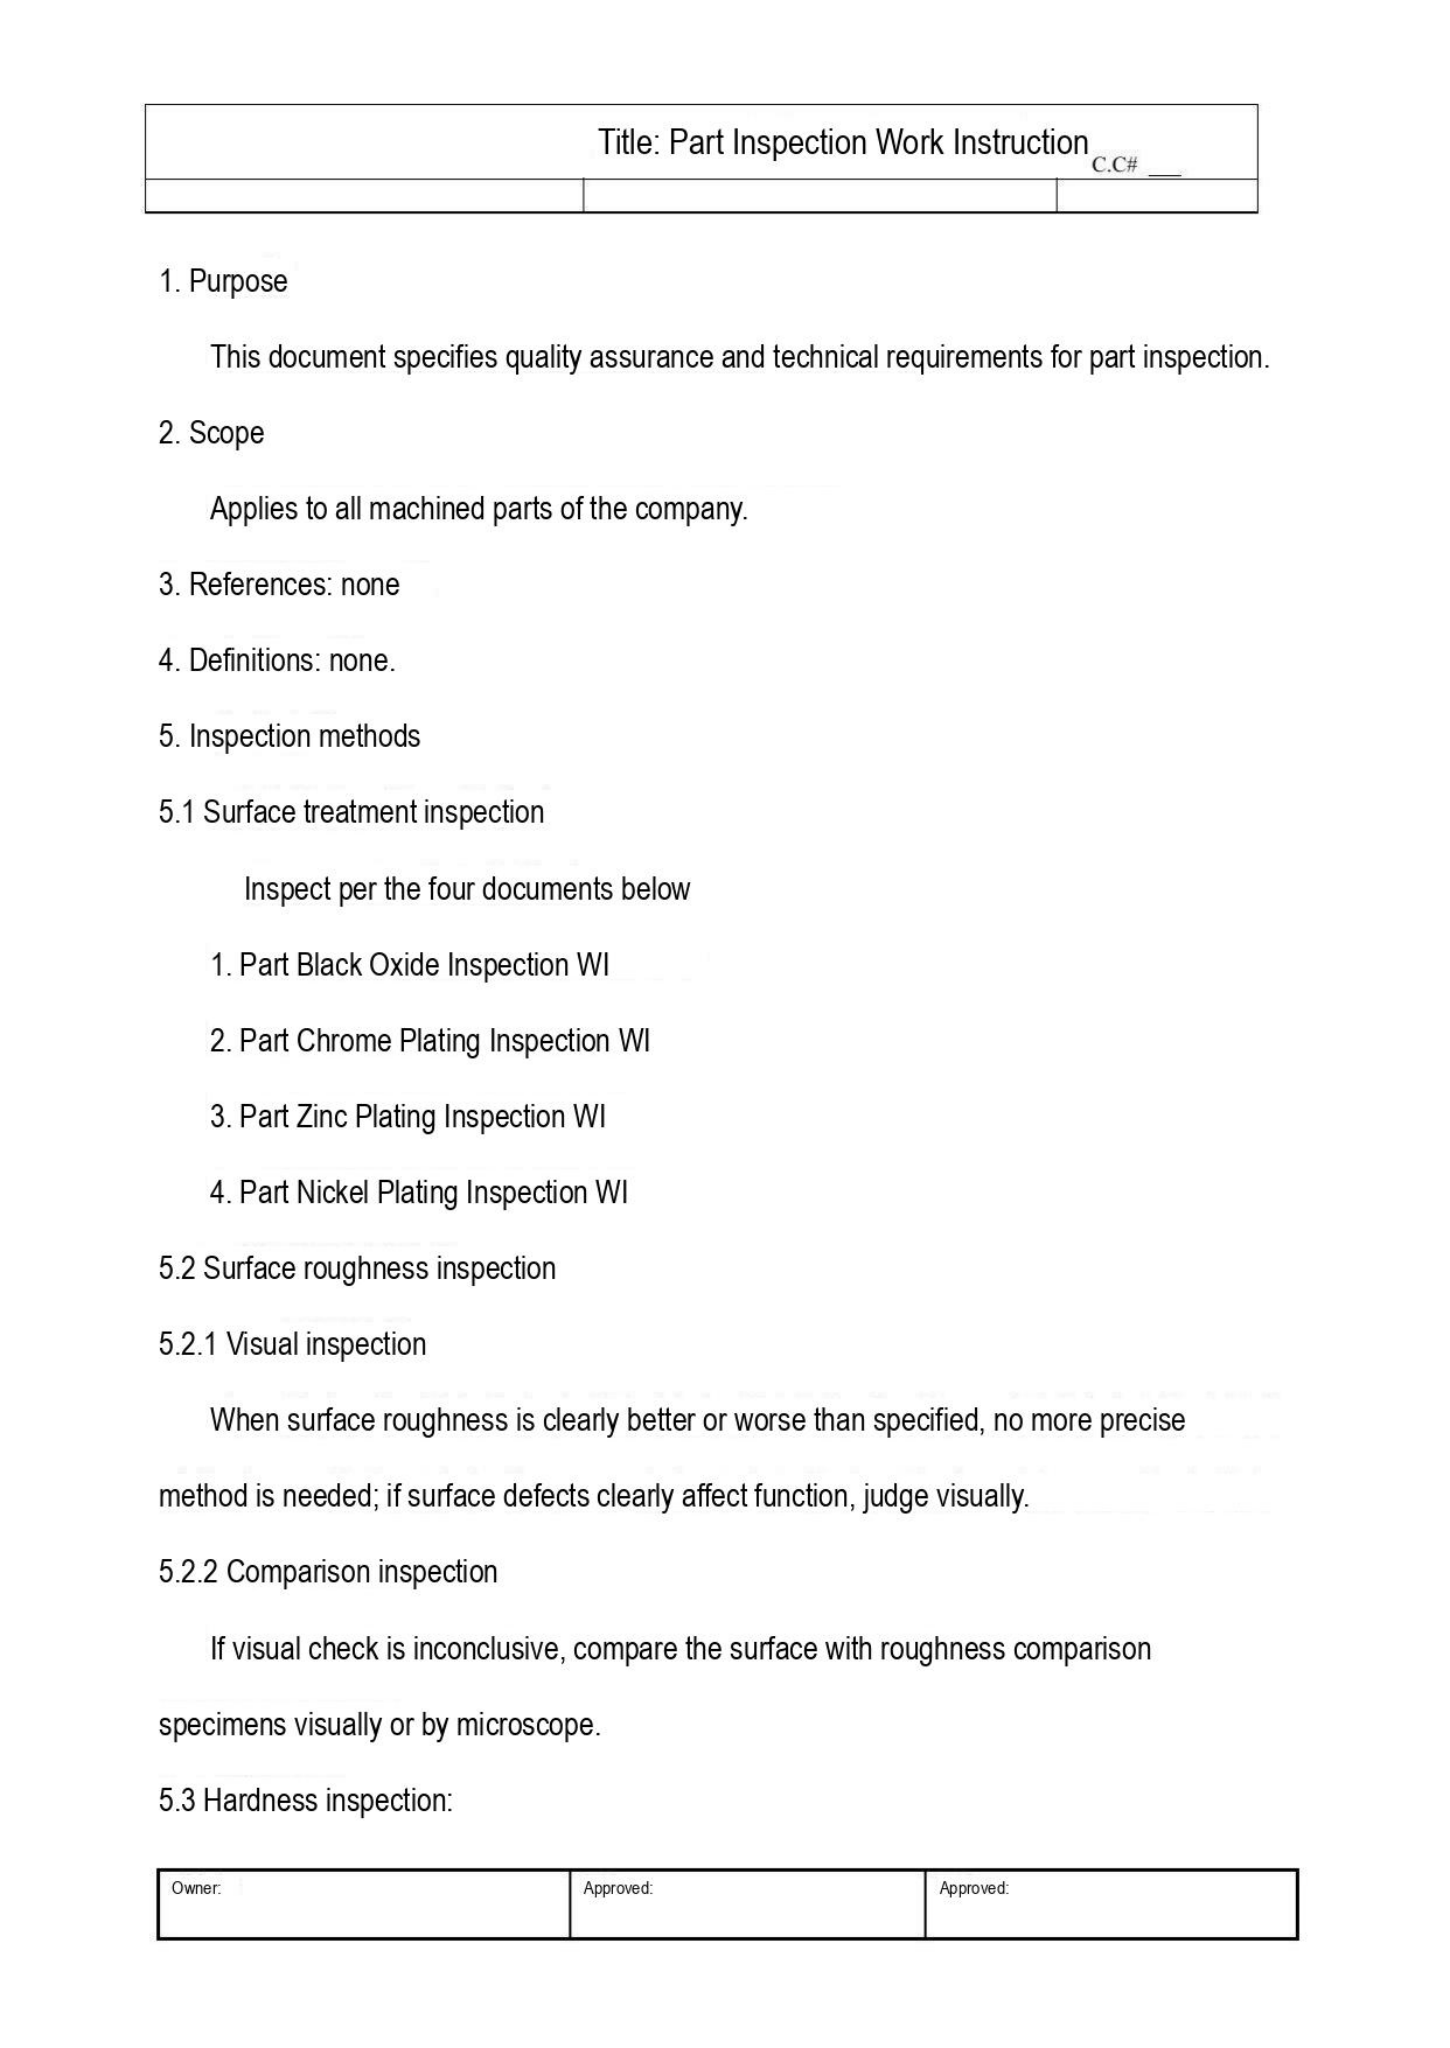| Title: Part Inspection Work Instruction C.C# ___ | | |
|---|---|---|
| | | |

1. Purpose

This document specifies quality assurance and technical requirements for part inspection.

2. Scope

Applies to all machined parts of the company.

3. References: none

4. Definitions: none.

5. Inspection methods

5.1 Surface treatment inspection

Inspect per the four documents below

1. Part Black Oxide Inspection WI

2. Part Chrome Plating Inspection WI

3. Part Zinc Plating Inspection WI

4. Part Nickel Plating Inspection WI

5.2 Surface roughness inspection

5.2.1 Visual inspection

When surface roughness is clearly better or worse than specified, no more precise method is needed; if surface defects clearly affect function, judge visually.

5.2.2 Comparison inspection

If visual check is inconclusive, compare the surface with roughness comparison specimens visually or by microscope.

5.3 Hardness inspection:

| Owner: | Approved: | Approved: |
|---|---|---|
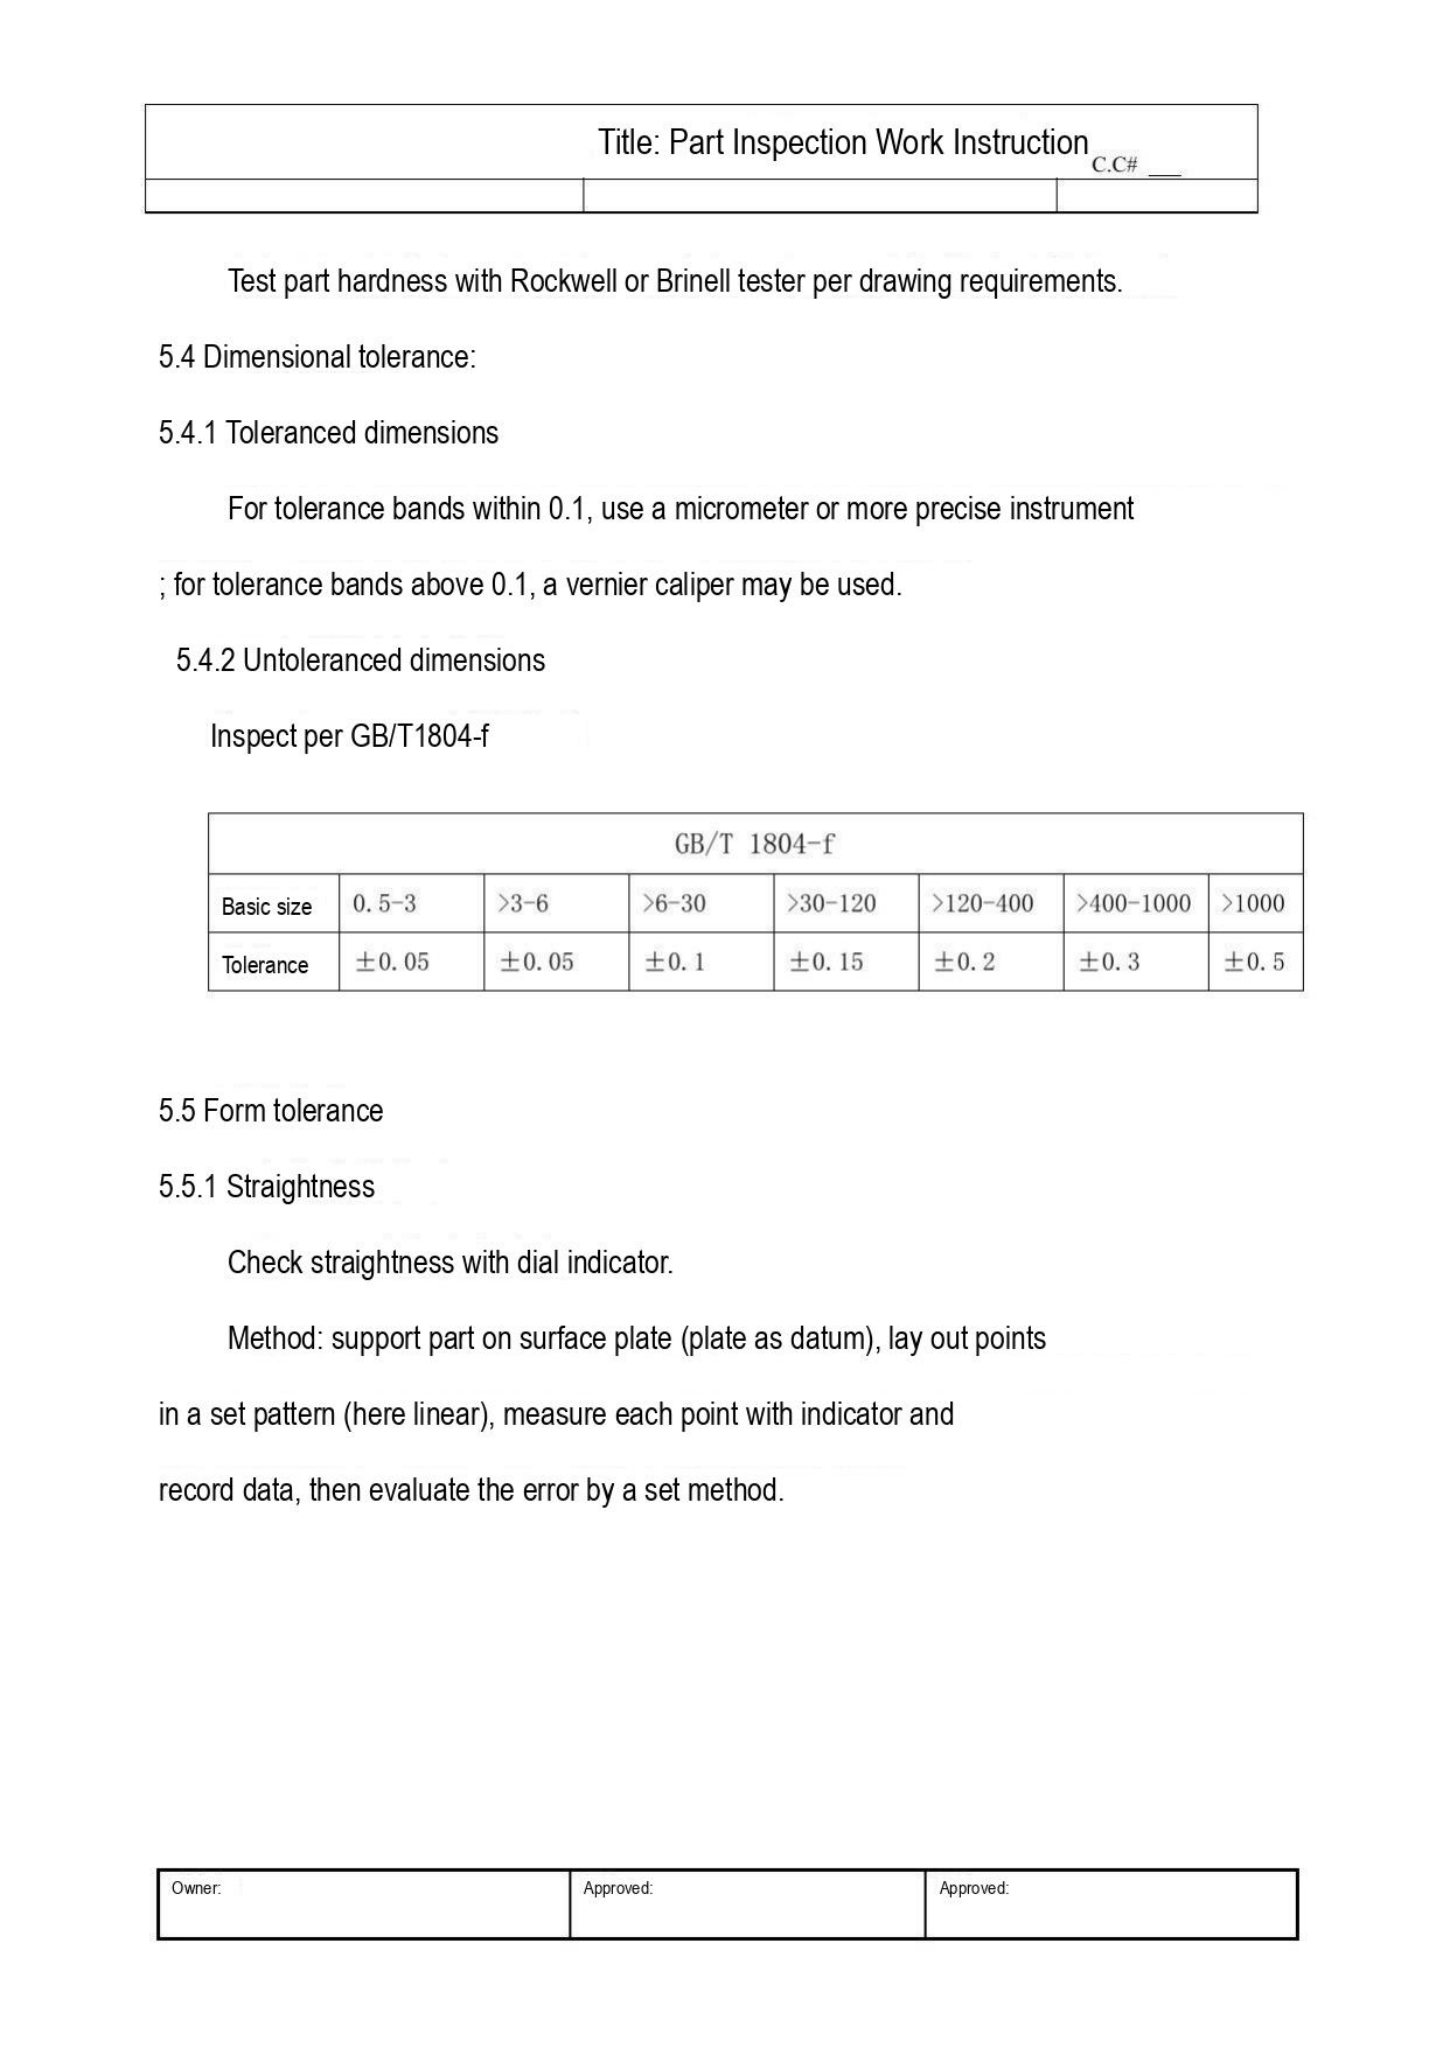Title: Part Inspection Work Instruction C.C# ___

Test part hardness with Rockwell or Brinell tester per drawing requirements.

5.4 Dimensional tolerance:

5.4.1 Toleranced dimensions

For tolerance bands within 0.1, use a micrometer or more precise instrument

; for tolerance bands above 0.1, a vernier caliper may be used.

5.4.2 Untoleranced dimensions

Inspect per GB/T1804-f

| GB/T 1804-f | | | | | | | |
|---|---|---|---|---|---|---|---|
| Basic size | 0. 5-3 | >3-6 | >6-30 | >30-120 | >120-400 | >400-1000 | >1000 |
| Tolerance | ±0. 05 | ±0. 05 | ±0. 1 | ±0. 15 | ±0. 2 | ±0. 3 | ±0. 5 |

5.5 Form tolerance

5.5.1 Straightness

Check straightness with dial indicator.

Method: support part on surface plate (plate as datum), lay out points

in a set pattern (here linear), measure each point with indicator and

record data, then evaluate the error by a set method.

| Owner: | Approved: | Approved: |
|---|---|---|
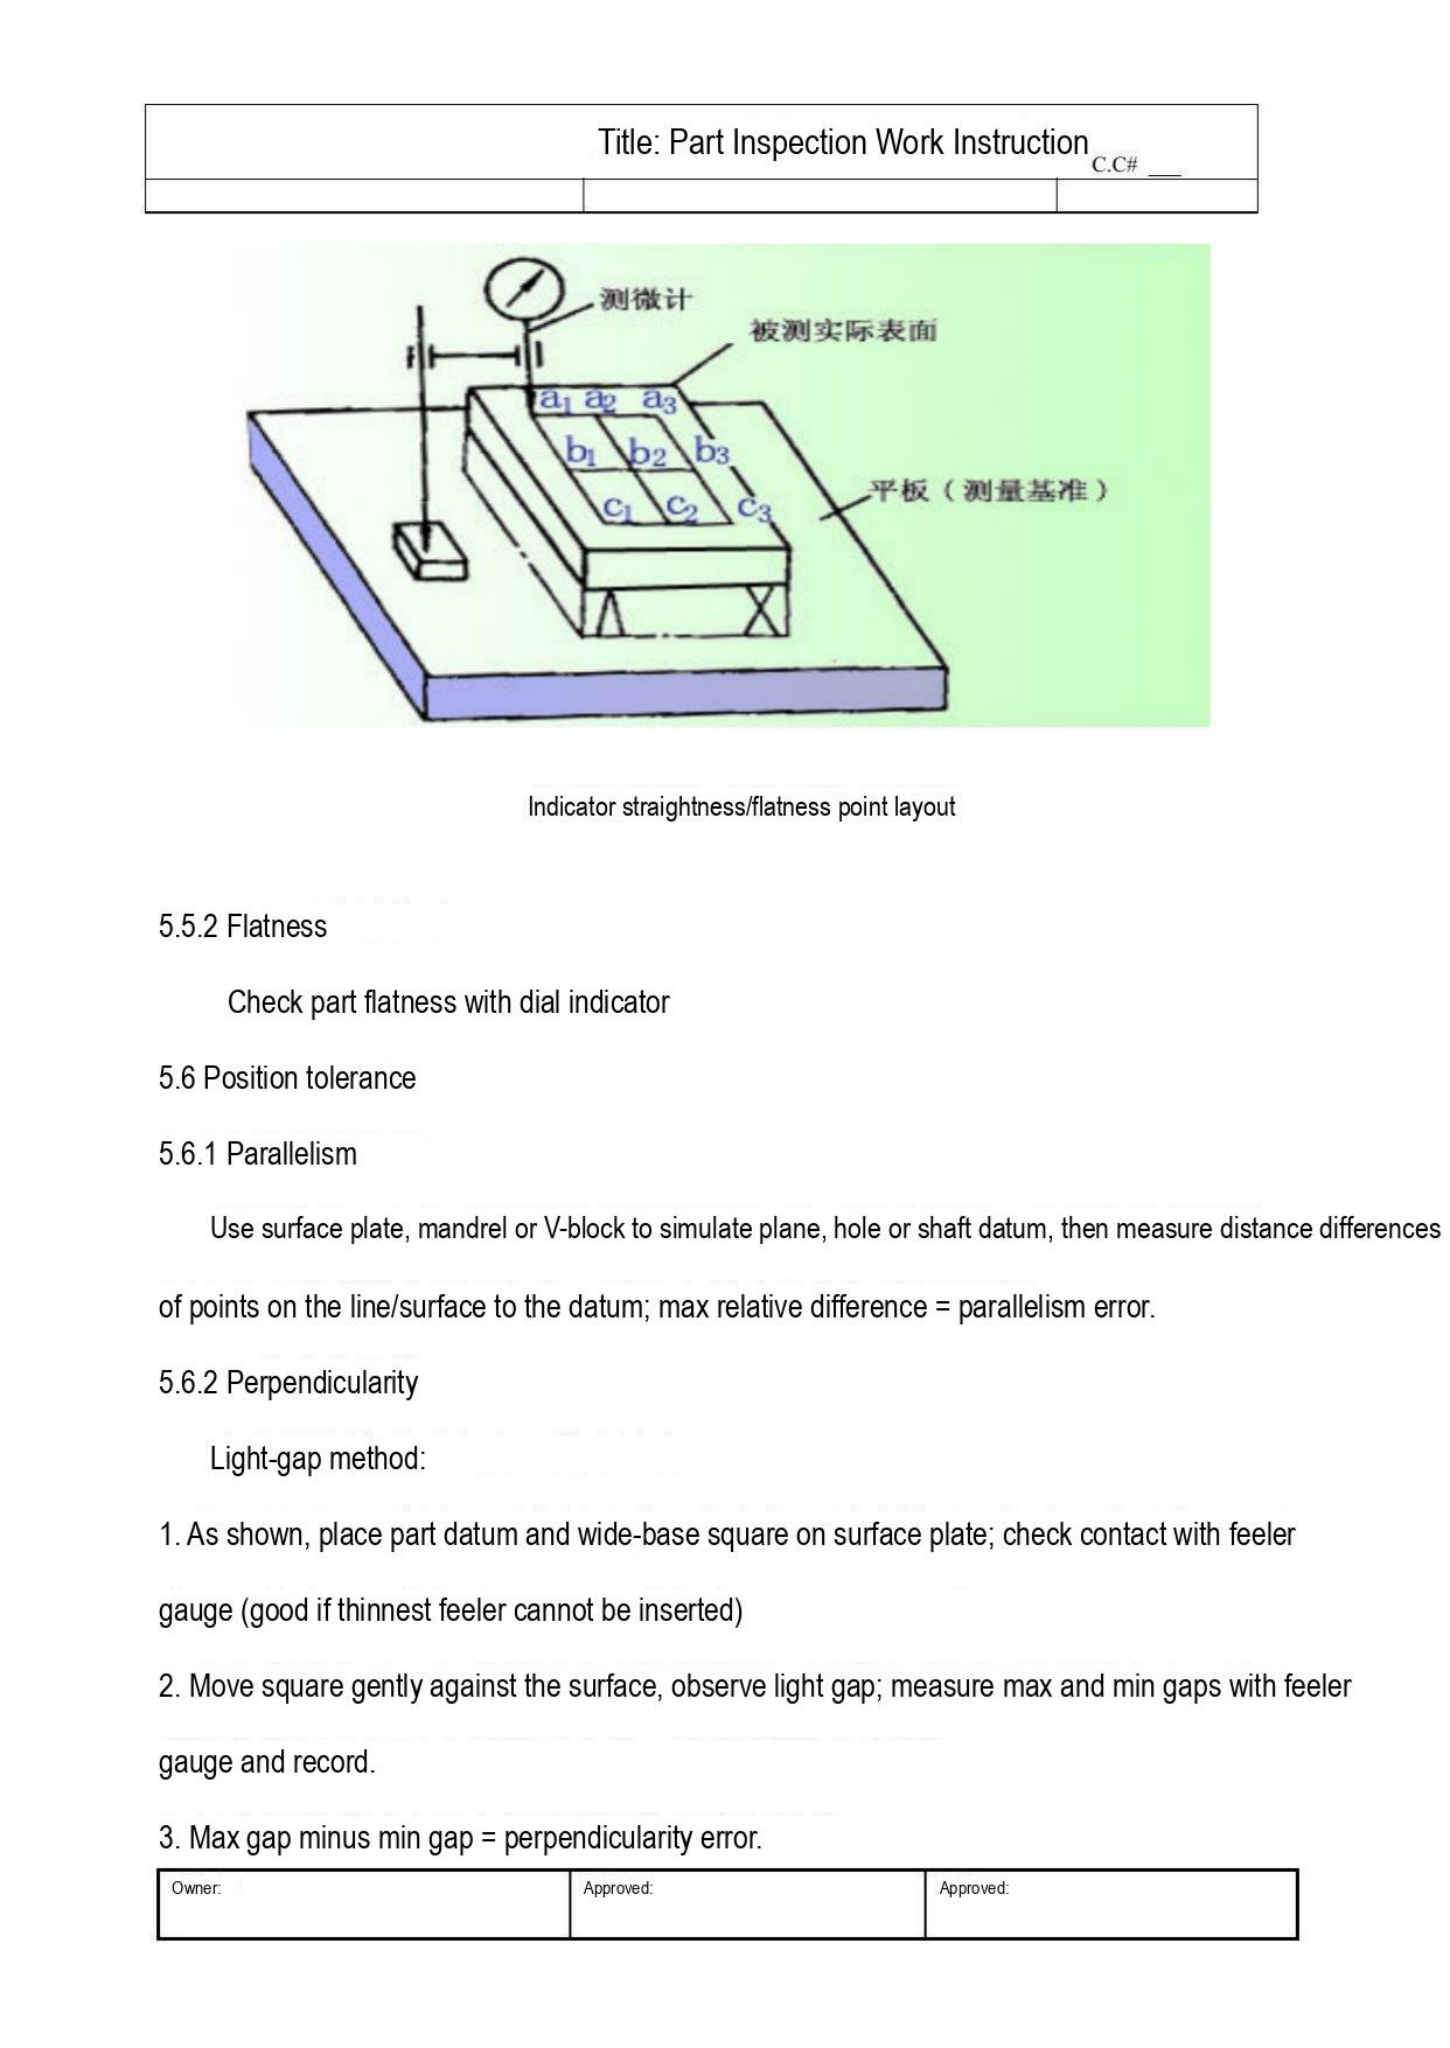| Title: Part Inspection Work Instruction C.C# ___ | | |
|---|---|---|
| | | |

测微计

被测实际表面

a1 a2 a3

b1 b2 b3

c1 c2 c3

平板（测量基准）

Indicator straightness/flatness point layout

5.5.2 Flatness

Check part flatness with dial indicator

5.6 Position tolerance

5.6.1 Parallelism

Use surface plate, mandrel or V-block to simulate plane, hole or shaft datum, then measure distance differences of points on the line/surface to the datum; max relative difference = parallelism error.

5.6.2 Perpendicularity

Light-gap method:

1. As shown, place part datum and wide-base square on surface plate; check contact with feeler gauge (good if thinnest feeler cannot be inserted)

2. Move square gently against the surface, observe light gap; measure max and min gaps with feeler gauge and record.

3. Max gap minus min gap = perpendicularity error.

| Owner: | Approved: | Approved: |
|---|---|---|
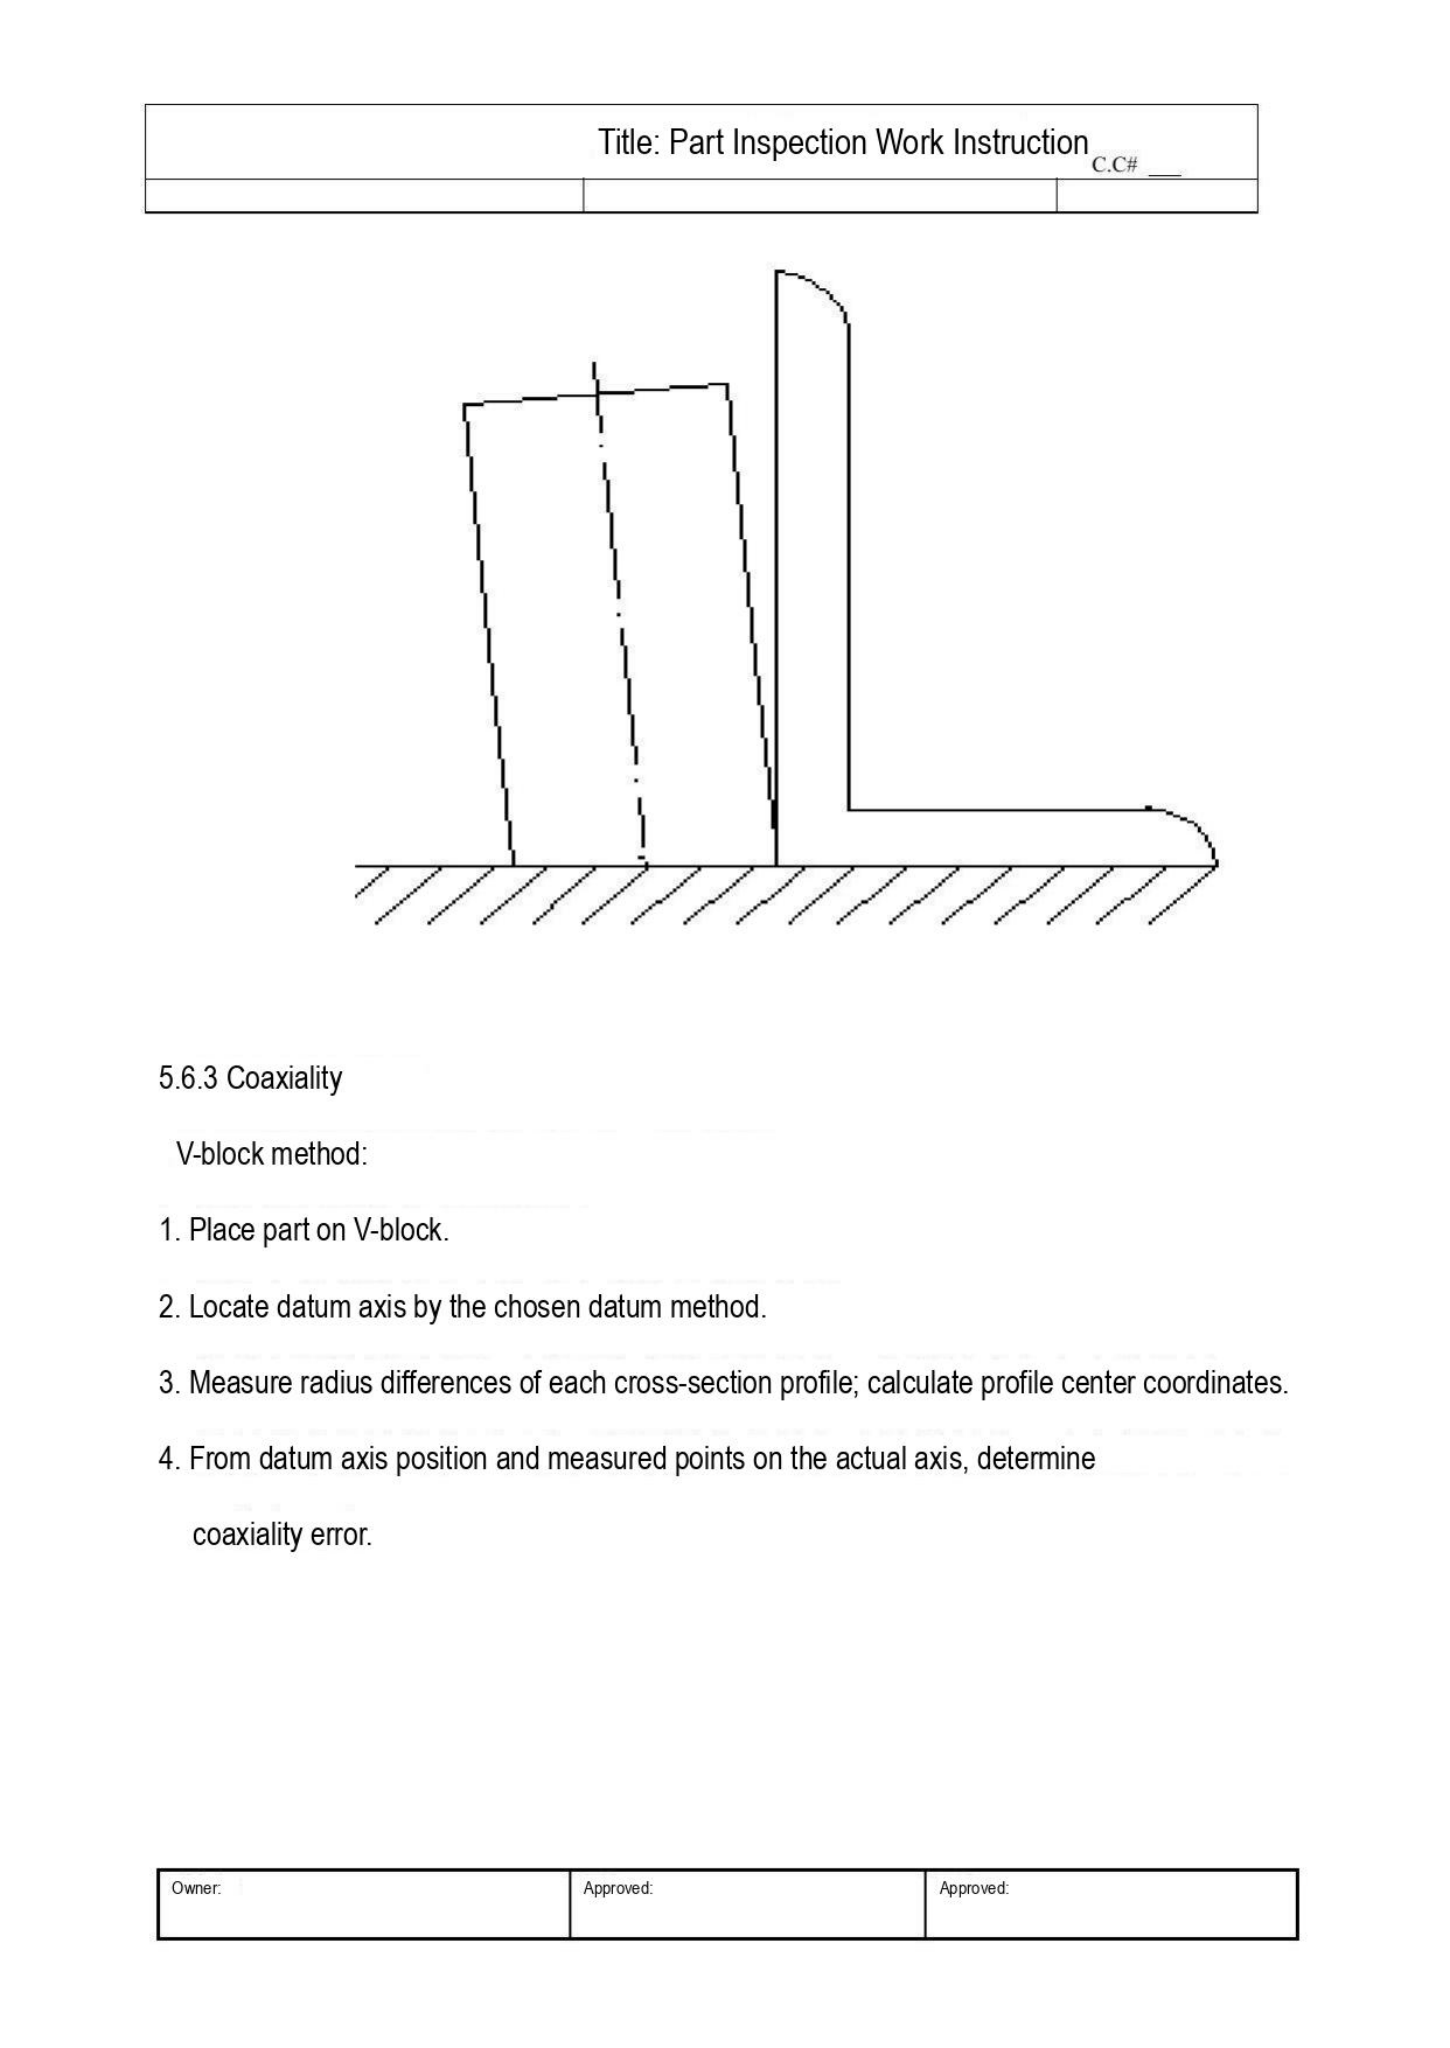Title: Part Inspection Work Instruction C.C# ___

5.6.3 Coaxiality

V-block method:

1. Place part on V-block.

2. Locate datum axis by the chosen datum method.

3. Measure radius differences of each cross-section profile; calculate profile center coordinates.

4. From datum axis position and measured points on the actual axis, determine coaxiality error.

| Owner: | Approved: | Approved: |
|---|---|---|
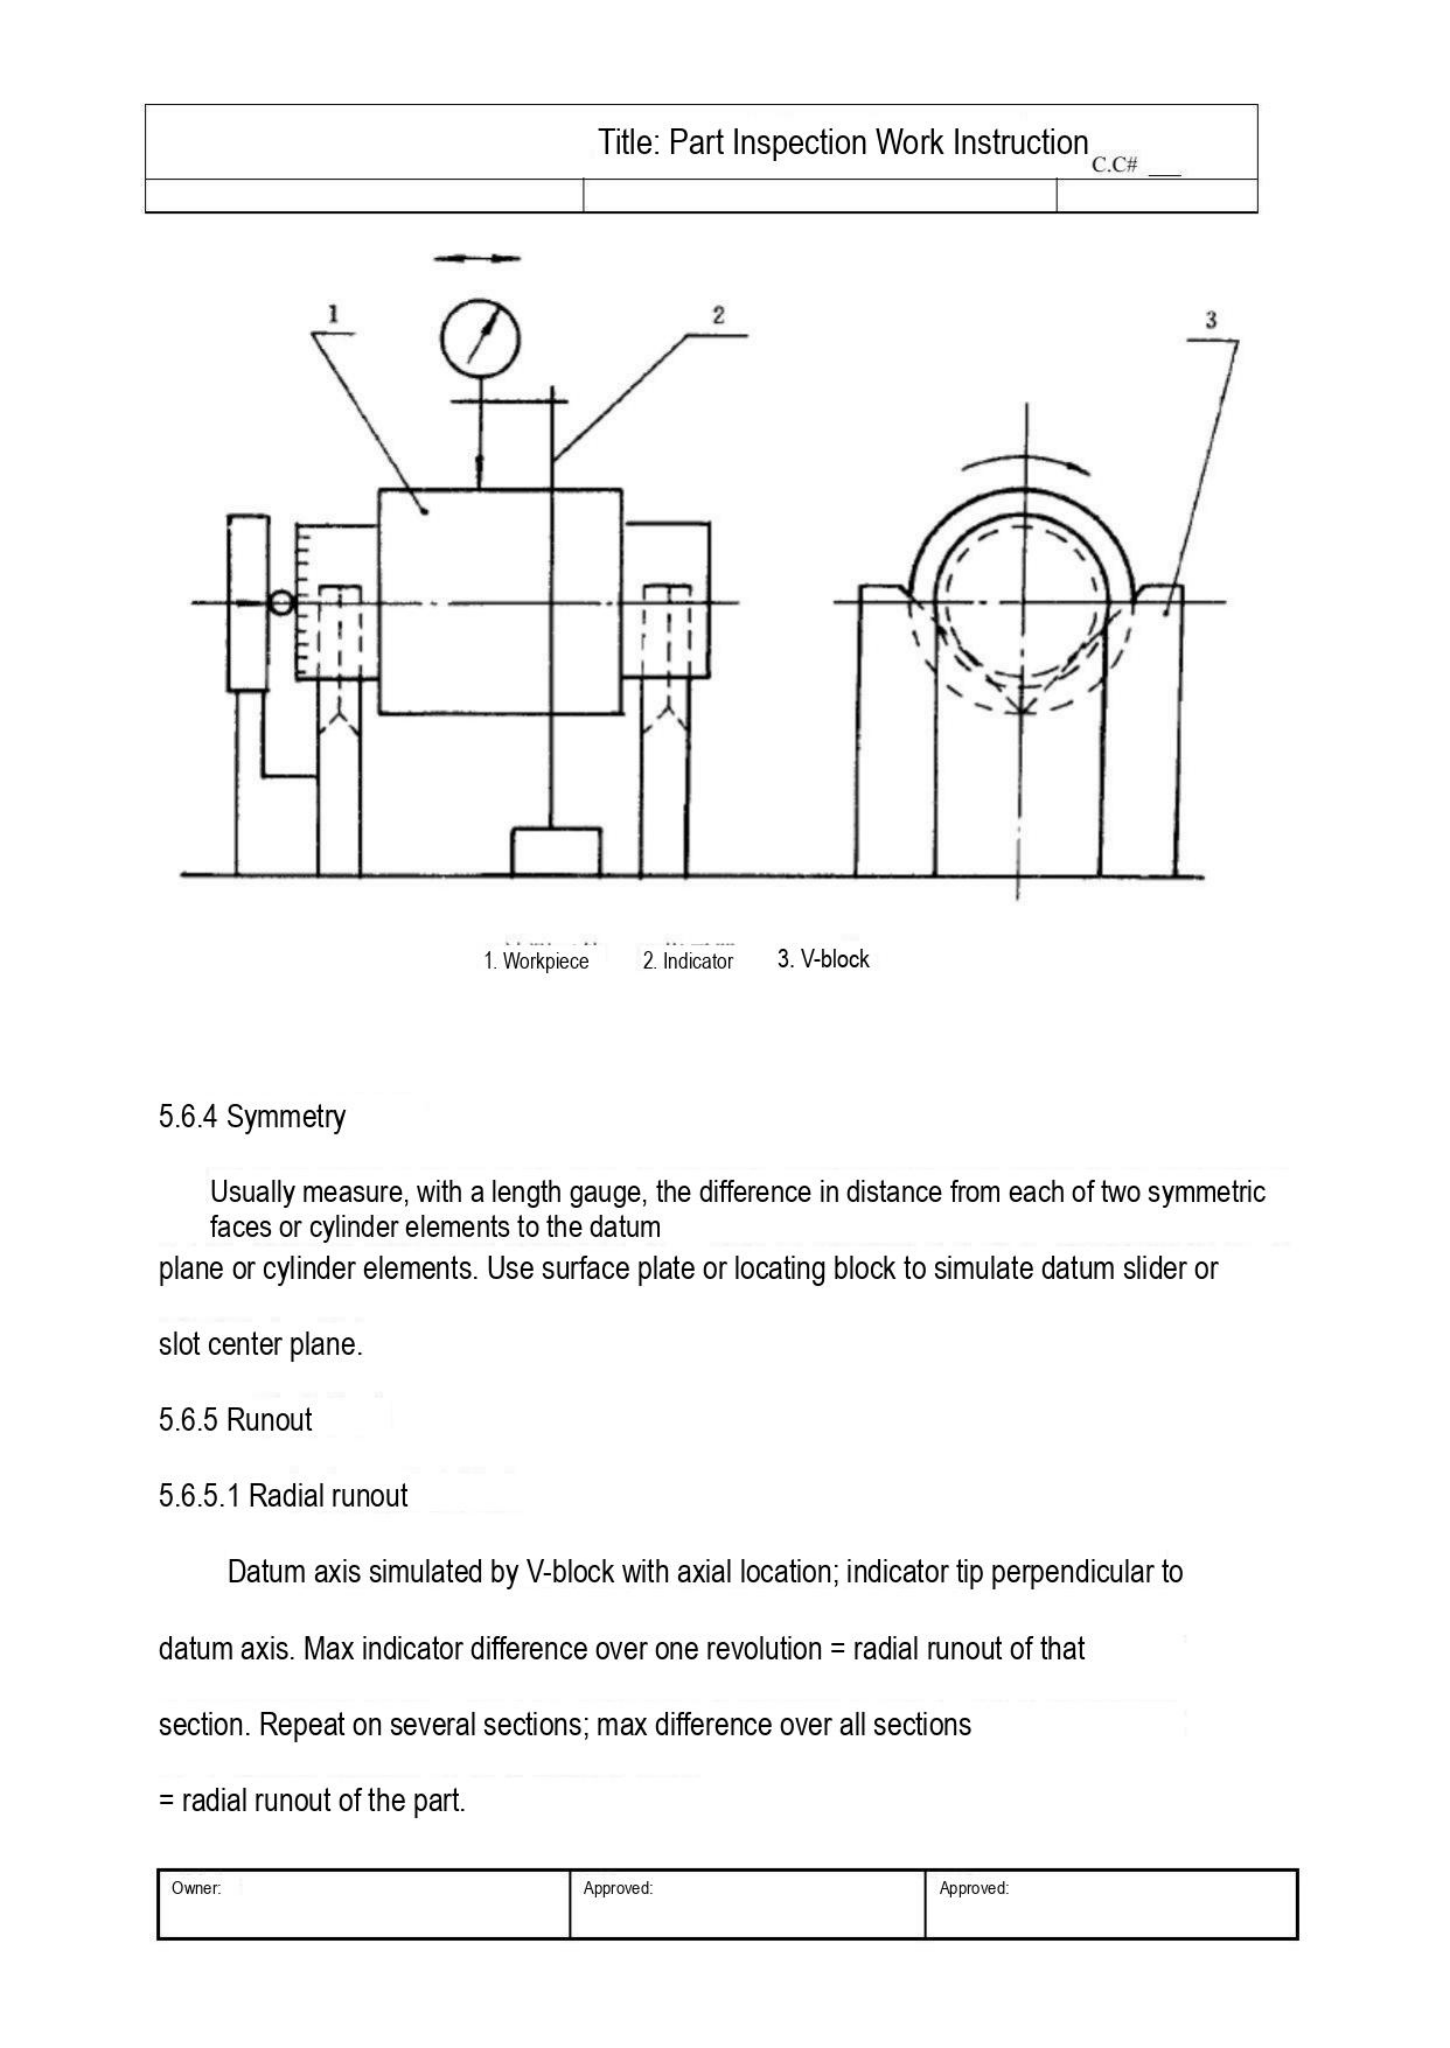| Title: Part Inspection Work Instruction C.C# ___ | | |
|---|---|---|
| | | |

1

2

3

1. Workpiece 2. Indicator 3. V-block

5.6.4 Symmetry

Usually measure, with a length gauge, the difference in distance from each of two symmetric faces or cylinder elements to the datum plane or cylinder elements. Use surface plate or locating block to simulate datum slider or slot center plane.

5.6.5 Runout

5.6.5.1 Radial runout

Datum axis simulated by V-block with axial location; indicator tip perpendicular to datum axis. Max indicator difference over one revolution = radial runout of that section. Repeat on several sections; max difference over all sections = radial runout of the part.

| Owner: | Approved: | Approved: |
|---|---|---|
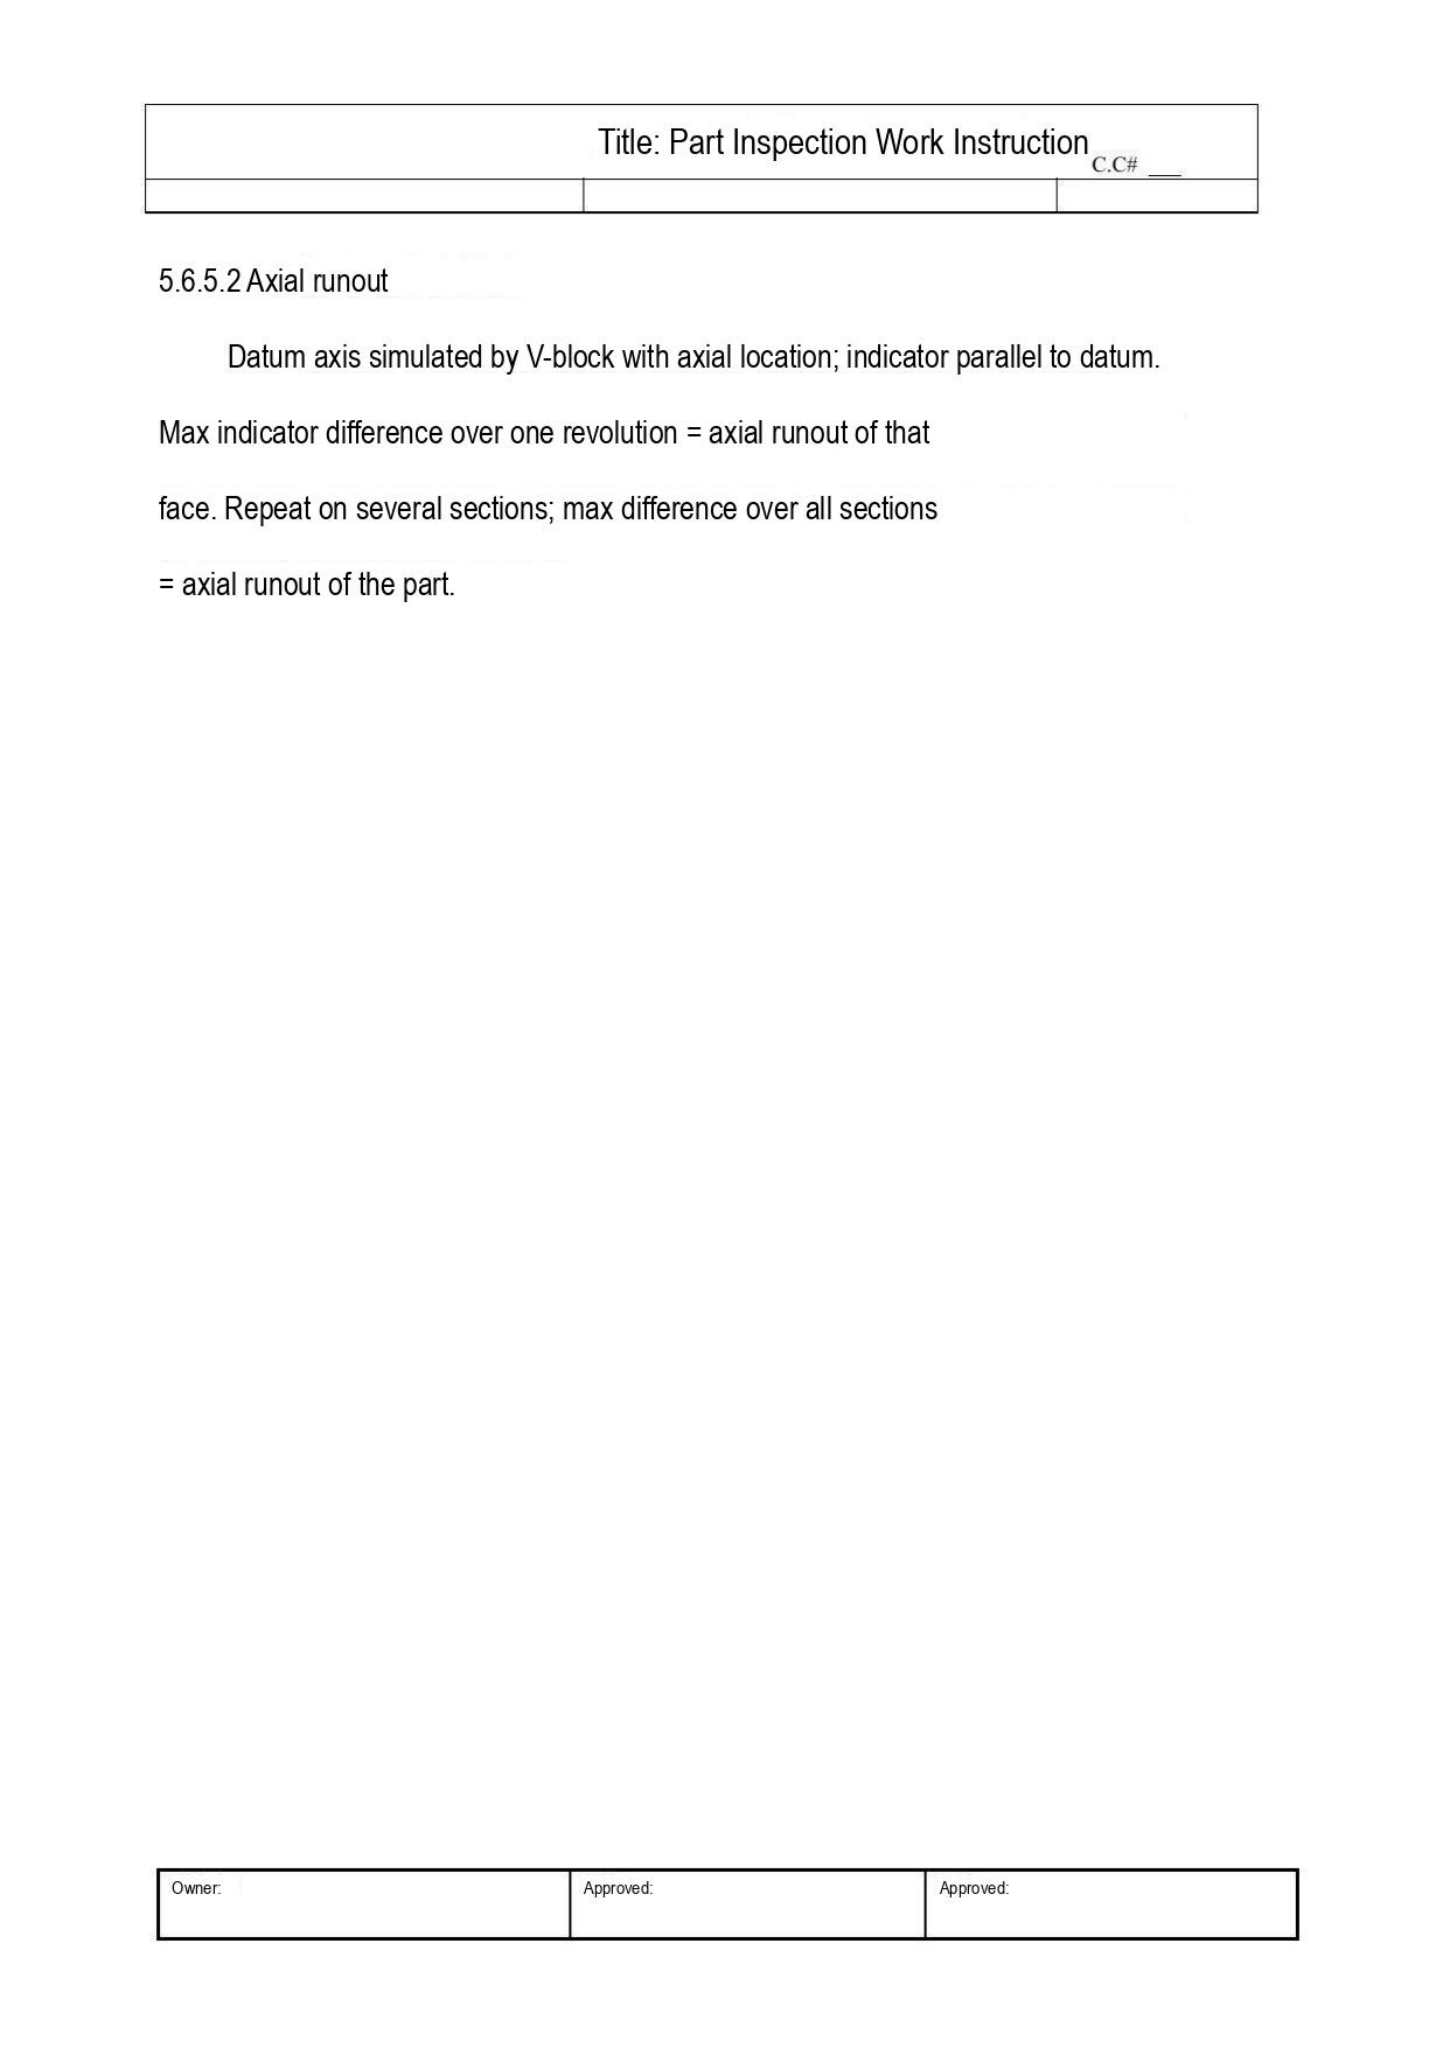Title: Part Inspection Work Instruction C.C# ___

5.6.5.2 Axial runout

Datum axis simulated by V-block with axial location; indicator parallel to datum. Max indicator difference over one revolution = axial runout of that face. Repeat on several sections; max difference over all sections = axial runout of the part.

| Owner: | Approved: | Approved: |
|---|---|---|